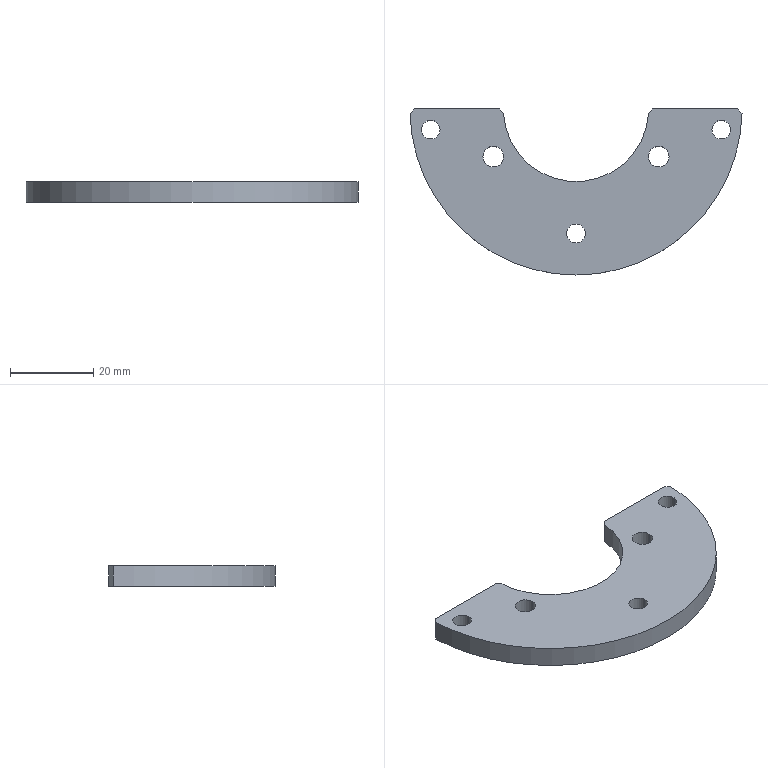Part | STEP file | End cover plate-lower | 1 solid | 20 faces | box 79.976 x 40 x 5 mm | volume 9716 mm3 | cylinder 12 | plane 8 | commonest cylinder face diameters 4.5 x6 5 x4 35 x1 80 x1